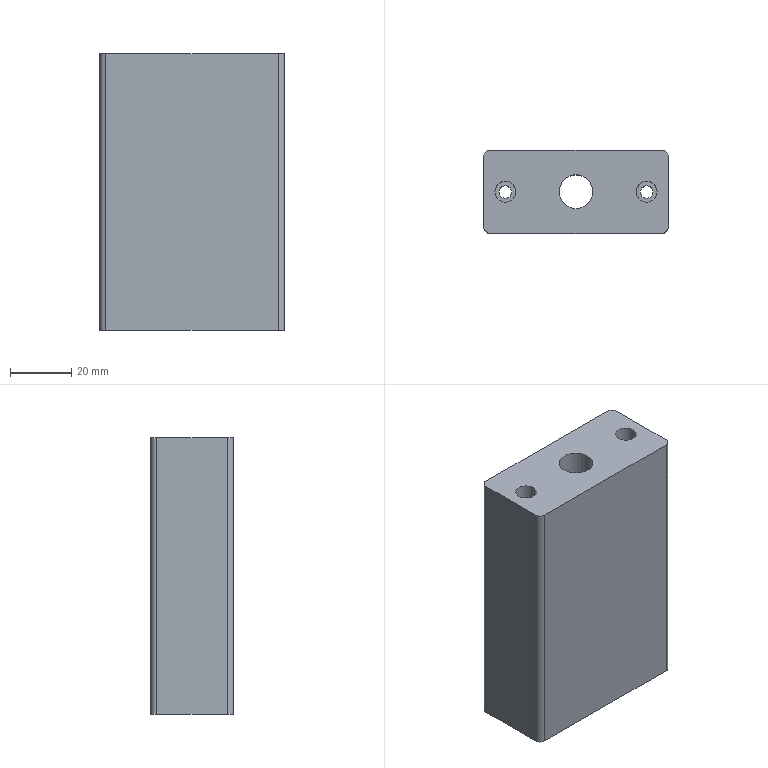Part | STEP file | gslz 2016.10.28-10_id2870_x_t | 1 solid | 19 faces | box 60 x 27 x 90 mm | volume 122829 mm3 | cylinder 10 | plane 9 | commonest cylinder face diameters 4 x4 4.1 x2 6.8 x2 11 x1 17 x1
STEP:
#1=CARTESIAN_POINT('',(0.,0.,0.));
#2=DIRECTION('',(0.,0.,1.));
#3=DIRECTION('',(1.,0.,0.));
#4=AXIS2_PLACEMENT_3D('',#1,#2,#3);
#5=CARTESIAN_POINT('',(1032.,147.5,85.));
#6=VERTEX_POINT('',#5);
#7=CARTESIAN_POINT('',(1088.,147.5,85.));
#8=VERTEX_POINT('',#7);
#9=CARTESIAN_POINT('',(1170.635,147.5,85.));
#10=DIRECTION('',(1.,0.,0.));
#11=VECTOR('',#10,1.);
#12=LINE('',#9,#11);
#13=CARTESIAN_POINT('',(1128.,155.,85.));
#14=DIRECTION('',(0.,0.,1.));
#15=DIRECTION('',(-1.,0.,0.));
#16=AXIS2_PLACEMENT_3D('',#13,#14,#15);
#17=PLANE('',#16);
#18=CARTESIAN_POINT('',(-42.635,7.5));
#19=DIRECTION('',(-1.,0.));
#20=VECTOR('',#19,1.);
#21=LINE('',#18,#20);
#22=(GEOMETRIC_REPRESENTATION_CONTEXT(2)PARAMETRIC_REPRESENTATION_CONTEXT()REPRESENTATION_CONTEXT('',''));
#23=DEFINITIONAL_REPRESENTATION('',(#21),#22);
#24=PCURVE('',#17,#23);
#25=CARTESIAN_POINT('',(1170.635,147.5,80.));
#26=DIRECTION('',(0.,1.,0.));
#27=DIRECTION('',(0.,0.,-1.));
#28=AXIS2_PLACEMENT_3D('',#25,#26,#27);
#29=PLANE('',#28);
#30=CARTESIAN_POINT('',(-5.,0.));
#31=DIRECTION('',(0.,-1.));
#32=VECTOR('',#31,1.);
#33=LINE('',#30,#32);
#34=(GEOMETRIC_REPRESENTATION_CONTEXT(2)PARAMETRIC_REPRESENTATION_CONTEXT()REPRESENTATION_CONTEXT('',''));
#35=DEFINITIONAL_REPRESENTATION('',(#33),#34);
#36=PCURVE('',#29,#35);
#37=SURFACE_CURVE('',#12,(#24,#36),.PCURVE_S1.);
#38=EDGE_CURVE('',#6,#8,#37,.T.);
#39=ORIENTED_EDGE('',*,*,#38,.T.);
#40=CARTESIAN_POINT('',(1090.,149.5,85.));
#41=VERTEX_POINT('',#40);
#42=CARTESIAN_POINT('',(1088.,149.5,85.));
#43=DIRECTION('',(0.,0.,1.));
#44=DIRECTION('',(1.,0.,0.));
#45=AXIS2_PLACEMENT_3D('',#42,#43,#44);
#46=CIRCLE('',#45,2.);
#47=CARTESIAN_POINT('',(40.,5.5));
#48=DIRECTION('',(-1.,0.));
#49=AXIS2_PLACEMENT_2D('',#47,#48);
#50=CIRCLE('',#49,2.);
#51=(GEOMETRIC_REPRESENTATION_CONTEXT(2)PARAMETRIC_REPRESENTATION_CONTEXT()REPRESENTATION_CONTEXT('',''));
#52=DEFINITIONAL_REPRESENTATION('',(#50),#51);
#53=PCURVE('',#17,#52);
#54=CARTESIAN_POINT('',(1088.,149.5,80.));
#55=DIRECTION('',(0.,0.,1.));
#56=DIRECTION('',(-1.,0.,0.));
#57=AXIS2_PLACEMENT_3D('',#54,#55,#56);
#58=CYLINDRICAL_SURFACE('',#57,2.);
#59=CARTESIAN_POINT('',(-3.142,5.));
#60=DIRECTION('',(1.,0.));
#61=VECTOR('',#60,1.);
#62=LINE('',#59,#61);
#63=(GEOMETRIC_REPRESENTATION_CONTEXT(2)PARAMETRIC_REPRESENTATION_CONTEXT()REPRESENTATION_CONTEXT('',''));
#64=DEFINITIONAL_REPRESENTATION('',(#62),#63);
#65=PCURVE('',#58,#64);
#66=SURFACE_CURVE('',#46,(#53,#65),.PCURVE_S1.);
#67=EDGE_CURVE('',#8,#41,#66,.T.);
#68=ORIENTED_EDGE('',*,*,#67,.T.);
#69=CARTESIAN_POINT('',(1090.,172.5,85.));
#70=VERTEX_POINT('',#69);
#71=CARTESIAN_POINT('',(1090.,161.,85.));
#72=DIRECTION('',(0.,1.,0.));
#73=VECTOR('',#72,1.);
#74=LINE('',#71,#73);
#75=CARTESIAN_POINT('',(38.,-6.));
#76=DIRECTION('',(0.,-1.));
#77=VECTOR('',#76,1.);
#78=LINE('',#75,#77);
#79=(GEOMETRIC_REPRESENTATION_CONTEXT(2)PARAMETRIC_REPRESENTATION_CONTEXT()REPRESENTATION_CONTEXT('',''));
#80=DEFINITIONAL_REPRESENTATION('',(#78),#79);
#81=PCURVE('',#17,#80);
#82=CARTESIAN_POINT('',(1090.,161.,46.));
#83=DIRECTION('',(-1.,0.,0.));
#84=DIRECTION('',(0.,0.,-1.));
#85=AXIS2_PLACEMENT_3D('',#82,#83,#84);
#86=PLANE('',#85);
#87=CARTESIAN_POINT('',(-39.,0.));
#88=DIRECTION('',(0.,-1.));
#89=VECTOR('',#88,1.);
#90=LINE('',#87,#89);
#91=(GEOMETRIC_REPRESENTATION_CONTEXT(2)PARAMETRIC_REPRESENTATION_CONTEXT()REPRESENTATION_CONTEXT('',''));
#92=DEFINITIONAL_REPRESENTATION('',(#90),#91);
#93=PCURVE('',#86,#92);
#94=SURFACE_CURVE('',#74,(#81,#93),.PCURVE_S1.);
#95=EDGE_CURVE('',#41,#70,#94,.T.);
#96=ORIENTED_EDGE('',*,*,#95,.T.);
#97=CARTESIAN_POINT('',(1088.,174.5,85.));
#98=VERTEX_POINT('',#97);
#99=CARTESIAN_POINT('',(1088.,172.5,85.));
#100=DIRECTION('',(0.,0.,1.));
#101=DIRECTION('',(1.,0.,0.));
#102=AXIS2_PLACEMENT_3D('',#99,#100,#101);
#103=CIRCLE('',#102,2.);
#104=CARTESIAN_POINT('',(40.,-17.5));
#105=DIRECTION('',(-1.,0.));
#106=AXIS2_PLACEMENT_2D('',#104,#105);
#107=CIRCLE('',#106,2.);
#108=(GEOMETRIC_REPRESENTATION_CONTEXT(2)PARAMETRIC_REPRESENTATION_CONTEXT()REPRESENTATION_CONTEXT('',''));
#109=DEFINITIONAL_REPRESENTATION('',(#107),#108);
#110=PCURVE('',#17,#109);
#111=CARTESIAN_POINT('',(1088.,172.5,46.));
#112=DIRECTION('',(0.,0.,1.));
#113=DIRECTION('',(-1.,0.,0.));
#114=AXIS2_PLACEMENT_3D('',#111,#112,#113);
#115=CYLINDRICAL_SURFACE('',#114,2.);
#116=CARTESIAN_POINT('',(-3.142,39.));
#117=DIRECTION('',(1.,0.));
#118=VECTOR('',#117,1.);
#119=LINE('',#116,#118);
#120=(GEOMETRIC_REPRESENTATION_CONTEXT(2)PARAMETRIC_REPRESENTATION_CONTEXT()REPRESENTATION_CONTEXT('',''));
#121=DEFINITIONAL_REPRESENTATION('',(#119),#120);
#122=PCURVE('',#115,#121);
#123=SURFACE_CURVE('',#103,(#110,#122),.PCURVE_S1.);
#124=EDGE_CURVE('',#70,#98,#123,.T.);
#125=ORIENTED_EDGE('',*,*,#124,.T.);
#126=CARTESIAN_POINT('',(1032.,174.5,85.));
#127=VERTEX_POINT('',#126);
#128=CARTESIAN_POINT('',(435.,174.5,85.));
#129=DIRECTION('',(-1.,0.,0.));
#130=VECTOR('',#129,1.);
#131=LINE('',#128,#130);
#132=CARTESIAN_POINT('',(693.,-19.5));
#133=DIRECTION('',(1.,0.));
#134=VECTOR('',#133,1.);
#135=LINE('',#132,#134);
#136=(GEOMETRIC_REPRESENTATION_CONTEXT(2)PARAMETRIC_REPRESENTATION_CONTEXT()REPRESENTATION_CONTEXT('',''));
#137=DEFINITIONAL_REPRESENTATION('',(#135),#136);
#138=PCURVE('',#17,#137);
#139=CARTESIAN_POINT('',(435.,174.5,80.));
#140=DIRECTION('',(0.,-1.,0.));
#141=DIRECTION('',(0.,0.,1.));
#142=AXIS2_PLACEMENT_3D('',#139,#140,#141);
#143=PLANE('',#142);
#144=CARTESIAN_POINT('',(5.,0.));
#145=DIRECTION('',(0.,1.));
#146=VECTOR('',#145,1.);
#147=LINE('',#144,#146);
#148=(GEOMETRIC_REPRESENTATION_CONTEXT(2)PARAMETRIC_REPRESENTATION_CONTEXT()REPRESENTATION_CONTEXT('',''));
#149=DEFINITIONAL_REPRESENTATION('',(#147),#148);
#150=PCURVE('',#143,#149);
#151=SURFACE_CURVE('',#131,(#138,#150),.PCURVE_S1.);
#152=EDGE_CURVE('',#98,#127,#151,.T.);
#153=ORIENTED_EDGE('',*,*,#152,.T.);
#154=CARTESIAN_POINT('',(1030.,172.5,85.));
#155=VERTEX_POINT('',#154);
#156=CARTESIAN_POINT('',(1032.,172.5,85.));
#157=DIRECTION('',(0.,0.,1.));
#158=DIRECTION('',(1.,0.,0.));
#159=AXIS2_PLACEMENT_3D('',#156,#157,#158);
#160=CIRCLE('',#159,2.);
#161=CARTESIAN_POINT('',(96.,-17.5));
#162=DIRECTION('',(-1.,0.));
#163=AXIS2_PLACEMENT_2D('',#161,#162);
#164=CIRCLE('',#163,2.);
#165=(GEOMETRIC_REPRESENTATION_CONTEXT(2)PARAMETRIC_REPRESENTATION_CONTEXT()REPRESENTATION_CONTEXT('',''));
#166=DEFINITIONAL_REPRESENTATION('',(#164),#165);
#167=PCURVE('',#17,#166);
#168=CARTESIAN_POINT('',(1032.,172.5,80.));
#169=DIRECTION('',(0.,0.,1.));
#170=DIRECTION('',(-1.,0.,0.));
#171=AXIS2_PLACEMENT_3D('',#168,#169,#170);
#172=CYLINDRICAL_SURFACE('',#171,2.);
#173=CARTESIAN_POINT('',(3.142,5.));
#174=DIRECTION('',(1.,0.));
#175=VECTOR('',#174,1.);
#176=LINE('',#173,#175);
#177=(GEOMETRIC_REPRESENTATION_CONTEXT(2)PARAMETRIC_REPRESENTATION_CONTEXT()REPRESENTATION_CONTEXT('',''));
#178=DEFINITIONAL_REPRESENTATION('',(#176),#177);
#179=PCURVE('',#172,#178);
#180=SURFACE_CURVE('',#160,(#167,#179),.PCURVE_S1.);
#181=EDGE_CURVE('',#127,#155,#180,.T.);
#182=ORIENTED_EDGE('',*,*,#181,.T.);
#183=CARTESIAN_POINT('',(1030.,149.5,85.));
#184=VERTEX_POINT('',#183);
#185=CARTESIAN_POINT('',(1030.,167.5,85.));
#186=DIRECTION('',(0.,1.,0.));
#187=VECTOR('',#186,1.);
#188=LINE('',#185,#187);
#189=CARTESIAN_POINT('',(98.,-12.5));
#190=DIRECTION('',(0.,-1.));
#191=VECTOR('',#190,1.);
#192=LINE('',#189,#191);
#193=(GEOMETRIC_REPRESENTATION_CONTEXT(2)PARAMETRIC_REPRESENTATION_CONTEXT()REPRESENTATION_CONTEXT('',''));
#194=DEFINITIONAL_REPRESENTATION('',(#192),#193);
#195=PCURVE('',#17,#194);
#196=CARTESIAN_POINT('',(1030.,167.5,80.));
#197=DIRECTION('',(-1.,0.,0.));
#198=DIRECTION('',(0.,0.,-1.));
#199=AXIS2_PLACEMENT_3D('',#196,#197,#198);
#200=PLANE('',#199);
#201=CARTESIAN_POINT('',(-5.,0.));
#202=DIRECTION('',(0.,-1.));
#203=VECTOR('',#202,1.);
#204=LINE('',#201,#203);
#205=(GEOMETRIC_REPRESENTATION_CONTEXT(2)PARAMETRIC_REPRESENTATION_CONTEXT()REPRESENTATION_CONTEXT('',''));
#206=DEFINITIONAL_REPRESENTATION('',(#204),#205);
#207=PCURVE('',#200,#206);
#208=SURFACE_CURVE('',#188,(#195,#207),.PCURVE_S1.);
#209=EDGE_CURVE('',#184,#155,#208,.T.);
#210=ORIENTED_EDGE('',*,*,#209,.F.);
#211=CARTESIAN_POINT('',(1032.,149.5,85.));
#212=DIRECTION('',(0.,0.,1.));
#213=DIRECTION('',(1.,0.,0.));
#214=AXIS2_PLACEMENT_3D('',#211,#212,#213);
#215=CIRCLE('',#214,2.);
#216=CARTESIAN_POINT('',(96.,5.5));
#217=DIRECTION('',(-1.,0.));
#218=AXIS2_PLACEMENT_2D('',#216,#217);
#219=CIRCLE('',#218,2.);
#220=(GEOMETRIC_REPRESENTATION_CONTEXT(2)PARAMETRIC_REPRESENTATION_CONTEXT()REPRESENTATION_CONTEXT('',''));
#221=DEFINITIONAL_REPRESENTATION('',(#219),#220);
#222=PCURVE('',#17,#221);
#223=CARTESIAN_POINT('',(1032.,149.5,80.));
#224=DIRECTION('',(0.,0.,1.));
#225=DIRECTION('',(-1.,0.,0.));
#226=AXIS2_PLACEMENT_3D('',#223,#224,#225);
#227=CYLINDRICAL_SURFACE('',#226,2.);
#228=CARTESIAN_POINT('',(-3.142,5.));
#229=DIRECTION('',(1.,0.));
#230=VECTOR('',#229,1.);
#231=LINE('',#228,#230);
#232=(GEOMETRIC_REPRESENTATION_CONTEXT(2)PARAMETRIC_REPRESENTATION_CONTEXT()REPRESENTATION_CONTEXT('',''));
#233=DEFINITIONAL_REPRESENTATION('',(#231),#232);
#234=PCURVE('',#227,#233);
#235=SURFACE_CURVE('',#215,(#222,#234),.PCURVE_S1.);
#236=EDGE_CURVE('',#184,#6,#235,.T.);
#237=ORIENTED_EDGE('',*,*,#236,.T.);
#238=EDGE_LOOP('',(#39,#68,#96,#125,#153,#182,#210,#237));
#239=FACE_BOUND('',#238,.T.);
#240=CARTESIAN_POINT('',(1065.5,161.,85.));
#241=VERTEX_POINT('',#240);
#242=CARTESIAN_POINT('',(1060.,161.,85.));
#243=DIRECTION('',(0.,0.,1.));
#244=DIRECTION('',(1.,0.,0.));
#245=AXIS2_PLACEMENT_3D('',#242,#243,#244);
#246=CIRCLE('',#245,5.5);
#247=CARTESIAN_POINT('',(68.,-6.));
#248=DIRECTION('',(-1.,0.));
#249=AXIS2_PLACEMENT_2D('',#247,#248);
#250=CIRCLE('',#249,5.5);
#251=(GEOMETRIC_REPRESENTATION_CONTEXT(2)PARAMETRIC_REPRESENTATION_CONTEXT()REPRESENTATION_CONTEXT('',''));
#252=DEFINITIONAL_REPRESENTATION('',(#250),#251);
#253=PCURVE('',#17,#252);
#254=CARTESIAN_POINT('',(1060.,161.,-13.));
#255=DIRECTION('',(0.,0.,1.));
#256=DIRECTION('',(1.,0.,0.));
#257=AXIS2_PLACEMENT_3D('',#254,#255,#256);
#258=CYLINDRICAL_SURFACE('',#257,5.5);
#259=CARTESIAN_POINT('',(0.,98.));
#260=DIRECTION('',(1.,0.));
#261=VECTOR('',#260,1.);
#262=LINE('',#259,#261);
#263=(GEOMETRIC_REPRESENTATION_CONTEXT(2)PARAMETRIC_REPRESENTATION_CONTEXT()REPRESENTATION_CONTEXT('',''));
#264=DEFINITIONAL_REPRESENTATION('',(#262),#263);
#265=PCURVE('',#258,#264);
#266=SURFACE_CURVE('',#246,(#253,#265),.PCURVE_S1.);
#267=EDGE_CURVE('',#241,#241,#266,.T.);
#268=ORIENTED_EDGE('',*,*,#267,.F.);
#269=EDGE_LOOP('',(#268));
#270=FACE_BOUND('',#269,.T.);
#271=CARTESIAN_POINT('',(1033.6,161.,85.));
#272=VERTEX_POINT('',#271);
#273=CARTESIAN_POINT('',(1037.,161.,85.));
#274=DIRECTION('',(0.,0.,1.));
#275=DIRECTION('',(-1.,0.,0.));
#276=AXIS2_PLACEMENT_3D('',#273,#274,#275);
#277=CIRCLE('',#276,3.4);
#278=CARTESIAN_POINT('',(91.,-6.));
#279=DIRECTION('',(1.,0.));
#280=AXIS2_PLACEMENT_2D('',#278,#279);
#281=CIRCLE('',#280,3.4);
#282=(GEOMETRIC_REPRESENTATION_CONTEXT(2)PARAMETRIC_REPRESENTATION_CONTEXT()REPRESENTATION_CONTEXT('',''));
#283=DEFINITIONAL_REPRESENTATION('',(#281),#282);
#284=PCURVE('',#17,#283);
#285=CARTESIAN_POINT('',(1037.,161.,31.));
#286=DIRECTION('',(0.,0.,1.));
#287=DIRECTION('',(1.,0.,0.));
#288=AXIS2_PLACEMENT_3D('',#285,#286,#287);
#289=CYLINDRICAL_SURFACE('',#288,3.4);
#290=CARTESIAN_POINT('',(3.142,54.));
#291=DIRECTION('',(1.,0.));
#292=VECTOR('',#291,1.);
#293=LINE('',#290,#292);
#294=(GEOMETRIC_REPRESENTATION_CONTEXT(2)PARAMETRIC_REPRESENTATION_CONTEXT()REPRESENTATION_CONTEXT('',''));
#295=DEFINITIONAL_REPRESENTATION('',(#293),#294);
#296=PCURVE('',#289,#295);
#297=SURFACE_CURVE('',#277,(#284,#296),.PCURVE_S1.);
#298=EDGE_CURVE('',#272,#272,#297,.T.);
#299=ORIENTED_EDGE('',*,*,#298,.F.);
#300=EDGE_LOOP('',(#299));
#301=FACE_BOUND('',#300,.T.);
#302=CARTESIAN_POINT('',(1086.4,161.,85.));
#303=VERTEX_POINT('',#302);
#304=CARTESIAN_POINT('',(1083.,161.,85.));
#305=DIRECTION('',(0.,0.,-1.));
#306=DIRECTION('',(1.,0.,0.));
#307=AXIS2_PLACEMENT_3D('',#304,#305,#306);
#308=CIRCLE('',#307,3.4);
#309=CARTESIAN_POINT('',(41.6,-6.));
#310=CARTESIAN_POINT('',(41.6,-0.111));
#311=CARTESIAN_POINT('',(46.7,-3.056));
#312=CARTESIAN_POINT('',(51.8,-6.));
#313=CARTESIAN_POINT('',(46.7,-8.944));
#314=CARTESIAN_POINT('',(41.6,-11.889));
#315=CARTESIAN_POINT('',(41.6,-6.));
#316=(BOUNDED_CURVE()B_SPLINE_CURVE(2,(#309,#310,#311,#312,#313,#314,#315),.UNSPECIFIED.,.T.,.F.)B_SPLINE_CURVE_WITH_KNOTS((1,2,2,2,2,1),(-2.094,0.,2.094,4.189,6.283,8.378),.UNSPECIFIED.)CURVE()GEOMETRIC_REPRESENTATION_ITEM()RATIONAL_B_SPLINE_CURVE((1.,0.5,1.,0.5,1.,0.5,1.))REPRESENTATION_ITEM(''));
#317=(GEOMETRIC_REPRESENTATION_CONTEXT(2)PARAMETRIC_REPRESENTATION_CONTEXT()REPRESENTATION_CONTEXT('',''));
#318=DEFINITIONAL_REPRESENTATION('',(#316),#317);
#319=PCURVE('',#17,#318);
#320=CARTESIAN_POINT('',(1083.,161.,31.));
#321=DIRECTION('',(0.,0.,1.));
#322=DIRECTION('',(-1.,0.,0.));
#323=AXIS2_PLACEMENT_3D('',#320,#321,#322);
#324=CYLINDRICAL_SURFACE('',#323,3.4);
#325=CARTESIAN_POINT('',(9.425,54.));
#326=DIRECTION('',(-1.,0.));
#327=VECTOR('',#326,1.);
#328=LINE('',#325,#327);
#329=(GEOMETRIC_REPRESENTATION_CONTEXT(2)PARAMETRIC_REPRESENTATION_CONTEXT()REPRESENTATION_CONTEXT('',''));
#330=DEFINITIONAL_REPRESENTATION('',(#328),#329);
#331=PCURVE('',#324,#330);
#332=SURFACE_CURVE('',#308,(#319,#331),.PCURVE_S1.);
#333=EDGE_CURVE('',#303,#303,#332,.T.);
#334=ORIENTED_EDGE('',*,*,#333,.T.);
#335=EDGE_LOOP('',(#334));
#336=FACE_BOUND('',#335,.T.);
#337=ADVANCED_FACE('',(#239,#270,#301,#336),#17,.T.);
#338=CARTESIAN_POINT('',(1080.95,161.,-5.));
#339=VERTEX_POINT('',#338);
#340=CARTESIAN_POINT('',(1083.,161.,-5.));
#341=DIRECTION('',(0.,0.,1.));
#342=DIRECTION('',(-1.,0.,0.));
#343=AXIS2_PLACEMENT_3D('',#340,#341,#342);
#344=CIRCLE('',#343,2.05);
#345=CARTESIAN_POINT('',(439.5,67.646,-5.));
#346=DIRECTION('',(0.,0.,-1.));
#347=DIRECTION('',(1.,0.,0.));
#348=AXIS2_PLACEMENT_3D('',#345,#346,#347);
#349=PLANE('',#348);
#350=CARTESIAN_POINT('',(641.45,-93.354));
#351=CARTESIAN_POINT('',(641.45,-89.804));
#352=CARTESIAN_POINT('',(644.525,-91.579));
#353=CARTESIAN_POINT('',(647.6,-93.354));
#354=CARTESIAN_POINT('',(644.525,-95.13));
#355=CARTESIAN_POINT('',(641.45,-96.905));
#356=CARTESIAN_POINT('',(641.45,-93.354));
#357=(BOUNDED_CURVE()B_SPLINE_CURVE(2,(#350,#351,#352,#353,#354,#355,#356),.UNSPECIFIED.,.T.,.F.)B_SPLINE_CURVE_WITH_KNOTS((1,2,2,2,2,1),(-2.094,0.,2.094,4.189,6.283,8.378),.UNSPECIFIED.)CURVE()GEOMETRIC_REPRESENTATION_ITEM()RATIONAL_B_SPLINE_CURVE((1.,0.5,1.,0.5,1.,0.5,1.))REPRESENTATION_ITEM(''));
#358=(GEOMETRIC_REPRESENTATION_CONTEXT(2)PARAMETRIC_REPRESENTATION_CONTEXT()REPRESENTATION_CONTEXT('',''));
#359=DEFINITIONAL_REPRESENTATION('',(#357),#358);
#360=PCURVE('',#349,#359);
#361=CARTESIAN_POINT('',(1083.,161.,36.));
#362=DIRECTION('',(0.,0.,-1.));
#363=DIRECTION('',(1.,0.,0.));
#364=AXIS2_PLACEMENT_3D('',#361,#362,#363);
#365=CYLINDRICAL_SURFACE('',#364,2.05);
#366=CARTESIAN_POINT('',(9.425,41.));
#367=DIRECTION('',(-1.,0.));
#368=VECTOR('',#367,1.);
#369=LINE('',#366,#368);
#370=(GEOMETRIC_REPRESENTATION_CONTEXT(2)PARAMETRIC_REPRESENTATION_CONTEXT()REPRESENTATION_CONTEXT('',''));
#371=DEFINITIONAL_REPRESENTATION('',(#369),#370);
#372=PCURVE('',#365,#371);
#373=SURFACE_CURVE('',#344,(#360,#372),.PCURVE_S1.);
#374=EDGE_CURVE('',#339,#339,#373,.T.);
#375=ORIENTED_EDGE('',*,*,#374,.T.);
#376=EDGE_LOOP('',(#375));
#377=FACE_BOUND('',#376,.T.);
#378=CARTESIAN_POINT('',(1034.95,161.,-5.));
#379=VERTEX_POINT('',#378);
#380=CARTESIAN_POINT('',(1037.,161.,-5.));
#381=DIRECTION('',(0.,0.,1.));
#382=DIRECTION('',(-1.,0.,0.));
#383=AXIS2_PLACEMENT_3D('',#380,#381,#382);
#384=CIRCLE('',#383,2.05);
#385=CARTESIAN_POINT('',(595.45,-93.354));
#386=CARTESIAN_POINT('',(595.45,-89.804));
#387=CARTESIAN_POINT('',(598.525,-91.579));
#388=CARTESIAN_POINT('',(601.6,-93.354));
#389=CARTESIAN_POINT('',(598.525,-95.13));
#390=CARTESIAN_POINT('',(595.45,-96.905));
#391=CARTESIAN_POINT('',(595.45,-93.354));
#392=(BOUNDED_CURVE()B_SPLINE_CURVE(2,(#385,#386,#387,#388,#389,#390,#391),.UNSPECIFIED.,.T.,.F.)B_SPLINE_CURVE_WITH_KNOTS((1,2,2,2,2,1),(-2.094,0.,2.094,4.189,6.283,8.378),.UNSPECIFIED.)CURVE()GEOMETRIC_REPRESENTATION_ITEM()RATIONAL_B_SPLINE_CURVE((1.,0.5,1.,0.5,1.,0.5,1.))REPRESENTATION_ITEM(''));
#393=(GEOMETRIC_REPRESENTATION_CONTEXT(2)PARAMETRIC_REPRESENTATION_CONTEXT()REPRESENTATION_CONTEXT('',''));
#394=DEFINITIONAL_REPRESENTATION('',(#392),#393);
#395=PCURVE('',#349,#394);
#396=CARTESIAN_POINT('',(1037.,161.,36.));
#397=DIRECTION('',(0.,0.,-1.));
#398=DIRECTION('',(-1.,0.,0.));
#399=AXIS2_PLACEMENT_3D('',#396,#397,#398);
#400=CYLINDRICAL_SURFACE('',#399,2.05);
#401=CARTESIAN_POINT('',(6.283,41.));
#402=DIRECTION('',(-1.,0.));
#403=VECTOR('',#402,1.);
#404=LINE('',#401,#403);
#405=(GEOMETRIC_REPRESENTATION_CONTEXT(2)PARAMETRIC_REPRESENTATION_CONTEXT()REPRESENTATION_CONTEXT('',''));
#406=DEFINITIONAL_REPRESENTATION('',(#404),#405);
#407=PCURVE('',#400,#406);
#408=SURFACE_CURVE('',#384,(#395,#407),.PCURVE_S1.);
#409=EDGE_CURVE('',#379,#379,#408,.T.);
#410=ORIENTED_EDGE('',*,*,#409,.T.);
#411=EDGE_LOOP('',(#410));
#412=FACE_BOUND('',#411,.T.);
#413=CARTESIAN_POINT('',(1090.,172.5,-5.));
#414=VERTEX_POINT('',#413);
#415=CARTESIAN_POINT('',(1090.,149.5,-5.));
#416=VERTEX_POINT('',#415);
#417=CARTESIAN_POINT('',(1090.,161.,-5.));
#418=DIRECTION('',(0.,-1.,0.));
#419=VECTOR('',#418,1.);
#420=LINE('',#417,#419);
#421=CARTESIAN_POINT('',(650.5,-93.354));
#422=DIRECTION('',(0.,1.));
#423=VECTOR('',#422,1.);
#424=LINE('',#421,#423);
#425=(GEOMETRIC_REPRESENTATION_CONTEXT(2)PARAMETRIC_REPRESENTATION_CONTEXT()REPRESENTATION_CONTEXT('',''));
#426=DEFINITIONAL_REPRESENTATION('',(#424),#425);
#427=PCURVE('',#349,#426);
#428=CARTESIAN_POINT('',(51.,0.));
#429=DIRECTION('',(0.,1.));
#430=VECTOR('',#429,1.);
#431=LINE('',#428,#430);
#432=(GEOMETRIC_REPRESENTATION_CONTEXT(2)PARAMETRIC_REPRESENTATION_CONTEXT()REPRESENTATION_CONTEXT('',''));
#433=DEFINITIONAL_REPRESENTATION('',(#431),#432);
#434=PCURVE('',#86,#433);
#435=SURFACE_CURVE('',#420,(#427,#434),.PCURVE_S1.);
#436=EDGE_CURVE('',#414,#416,#435,.T.);
#437=ORIENTED_EDGE('',*,*,#436,.T.);
#438=CARTESIAN_POINT('',(1088.,147.5,-5.));
#439=VERTEX_POINT('',#438);
#440=CARTESIAN_POINT('',(1088.,149.5,-5.));
#441=DIRECTION('',(0.,0.,-1.));
#442=DIRECTION('',(-1.,0.,0.));
#443=AXIS2_PLACEMENT_3D('',#440,#441,#442);
#444=CIRCLE('',#443,2.);
#445=CARTESIAN_POINT('',(648.5,-81.854));
#446=DIRECTION('',(-1.,0.));
#447=AXIS2_PLACEMENT_2D('',#445,#446);
#448=CIRCLE('',#447,2.);
#449=(GEOMETRIC_REPRESENTATION_CONTEXT(2)PARAMETRIC_REPRESENTATION_CONTEXT()REPRESENTATION_CONTEXT('',''));
#450=DEFINITIONAL_REPRESENTATION('',(#448),#449);
#451=PCURVE('',#349,#450);
#452=CARTESIAN_POINT('',(6.283,-85.));
#453=DIRECTION('',(-1.,0.));
#454=VECTOR('',#453,1.);
#455=LINE('',#452,#454);
#456=(GEOMETRIC_REPRESENTATION_CONTEXT(2)PARAMETRIC_REPRESENTATION_CONTEXT()REPRESENTATION_CONTEXT('',''));
#457=DEFINITIONAL_REPRESENTATION('',(#455),#456);
#458=PCURVE('',#58,#457);
#459=SURFACE_CURVE('',#444,(#451,#458),.PCURVE_S1.);
#460=EDGE_CURVE('',#416,#439,#459,.T.);
#461=ORIENTED_EDGE('',*,*,#460,.T.);
#462=CARTESIAN_POINT('',(1032.,147.5,-5.));
#463=VERTEX_POINT('',#462);
#464=CARTESIAN_POINT('',(439.5,147.5,-5.));
#465=DIRECTION('',(1.,0.,0.));
#466=VECTOR('',#465,1.);
#467=LINE('',#464,#466);
#468=CARTESIAN_POINT('',(0.,-79.854));
#469=DIRECTION('',(1.,0.));
#470=VECTOR('',#469,1.);
#471=LINE('',#468,#470);
#472=(GEOMETRIC_REPRESENTATION_CONTEXT(2)PARAMETRIC_REPRESENTATION_CONTEXT()REPRESENTATION_CONTEXT('',''));
#473=DEFINITIONAL_REPRESENTATION('',(#471),#472);
#474=PCURVE('',#349,#473);
#475=CARTESIAN_POINT('',(85.,731.135));
#476=DIRECTION('',(0.,-1.));
#477=VECTOR('',#476,1.);
#478=LINE('',#475,#477);
#479=(GEOMETRIC_REPRESENTATION_CONTEXT(2)PARAMETRIC_REPRESENTATION_CONTEXT()REPRESENTATION_CONTEXT('',''));
#480=DEFINITIONAL_REPRESENTATION('',(#478),#479);
#481=PCURVE('',#29,#480);
#482=SURFACE_CURVE('',#467,(#474,#481),.PCURVE_S1.);
#483=EDGE_CURVE('',#463,#439,#482,.T.);
#484=ORIENTED_EDGE('',*,*,#483,.F.);
#485=CARTESIAN_POINT('',(1030.,149.5,-5.));
#486=VERTEX_POINT('',#485);
#487=CARTESIAN_POINT('',(1032.,149.5,-5.));
#488=DIRECTION('',(0.,0.,-1.));
#489=DIRECTION('',(-1.,0.,0.));
#490=AXIS2_PLACEMENT_3D('',#487,#488,#489);
#491=CIRCLE('',#490,2.);
#492=CARTESIAN_POINT('',(592.5,-81.854));
#493=DIRECTION('',(-1.,0.));
#494=AXIS2_PLACEMENT_2D('',#492,#493);
#495=CIRCLE('',#494,2.);
#496=(GEOMETRIC_REPRESENTATION_CONTEXT(2)PARAMETRIC_REPRESENTATION_CONTEXT()REPRESENTATION_CONTEXT('',''));
#497=DEFINITIONAL_REPRESENTATION('',(#495),#496);
#498=PCURVE('',#349,#497);
#499=CARTESIAN_POINT('',(6.283,-85.));
#500=DIRECTION('',(-1.,0.));
#501=VECTOR('',#500,1.);
#502=LINE('',#499,#501);
#503=(GEOMETRIC_REPRESENTATION_CONTEXT(2)PARAMETRIC_REPRESENTATION_CONTEXT()REPRESENTATION_CONTEXT('',''));
#504=DEFINITIONAL_REPRESENTATION('',(#502),#503);
#505=PCURVE('',#227,#504);
#506=SURFACE_CURVE('',#491,(#498,#505),.PCURVE_S1.);
#507=EDGE_CURVE('',#463,#486,#506,.T.);
#508=ORIENTED_EDGE('',*,*,#507,.T.);
#509=CARTESIAN_POINT('',(1030.,172.5,-5.));
#510=VERTEX_POINT('',#509);
#511=CARTESIAN_POINT('',(1030.,67.646,-5.));
#512=DIRECTION('',(0.,1.,0.));
#513=VECTOR('',#512,1.);
#514=LINE('',#511,#513);
#515=CARTESIAN_POINT('',(590.5,0.));
#516=DIRECTION('',(0.,-1.));
#517=VECTOR('',#516,1.);
#518=LINE('',#515,#517);
#519=(GEOMETRIC_REPRESENTATION_CONTEXT(2)PARAMETRIC_REPRESENTATION_CONTEXT()REPRESENTATION_CONTEXT('',''));
#520=DEFINITIONAL_REPRESENTATION('',(#518),#519);
#521=PCURVE('',#349,#520);
#522=CARTESIAN_POINT('',(85.,99.854));
#523=DIRECTION('',(0.,-1.));
#524=VECTOR('',#523,1.);
#525=LINE('',#522,#524);
#526=(GEOMETRIC_REPRESENTATION_CONTEXT(2)PARAMETRIC_REPRESENTATION_CONTEXT()REPRESENTATION_CONTEXT('',''));
#527=DEFINITIONAL_REPRESENTATION('',(#525),#526);
#528=PCURVE('',#200,#527);
#529=SURFACE_CURVE('',#514,(#521,#528),.PCURVE_S1.);
#530=EDGE_CURVE('',#486,#510,#529,.T.);
#531=ORIENTED_EDGE('',*,*,#530,.T.);
#532=CARTESIAN_POINT('',(1032.,174.5,-5.));
#533=VERTEX_POINT('',#532);
#534=CARTESIAN_POINT('',(1032.,172.5,-5.));
#535=DIRECTION('',(0.,0.,-1.));
#536=DIRECTION('',(-1.,0.,0.));
#537=AXIS2_PLACEMENT_3D('',#534,#535,#536);
#538=CIRCLE('',#537,2.);
#539=CARTESIAN_POINT('',(592.5,-104.854));
#540=DIRECTION('',(-1.,0.));
#541=AXIS2_PLACEMENT_2D('',#539,#540);
#542=CIRCLE('',#541,2.);
#543=(GEOMETRIC_REPRESENTATION_CONTEXT(2)PARAMETRIC_REPRESENTATION_CONTEXT()REPRESENTATION_CONTEXT('',''));
#544=DEFINITIONAL_REPRESENTATION('',(#542),#543);
#545=PCURVE('',#349,#544);
#546=CARTESIAN_POINT('',(6.283,-85.));
#547=DIRECTION('',(-1.,0.));
#548=VECTOR('',#547,1.);
#549=LINE('',#546,#548);
#550=(GEOMETRIC_REPRESENTATION_CONTEXT(2)PARAMETRIC_REPRESENTATION_CONTEXT()REPRESENTATION_CONTEXT('',''));
#551=DEFINITIONAL_REPRESENTATION('',(#549),#550);
#552=PCURVE('',#172,#551);
#553=SURFACE_CURVE('',#538,(#545,#552),.PCURVE_S1.);
#554=EDGE_CURVE('',#510,#533,#553,.T.);
#555=ORIENTED_EDGE('',*,*,#554,.T.);
#556=CARTESIAN_POINT('',(1088.,174.5,-5.));
#557=VERTEX_POINT('',#556);
#558=CARTESIAN_POINT('',(439.5,174.5,-5.));
#559=DIRECTION('',(-1.,0.,0.));
#560=VECTOR('',#559,1.);
#561=LINE('',#558,#560);
#562=CARTESIAN_POINT('',(0.,-106.854));
#563=DIRECTION('',(-1.,0.));
#564=VECTOR('',#563,1.);
#565=LINE('',#562,#564);
#566=(GEOMETRIC_REPRESENTATION_CONTEXT(2)PARAMETRIC_REPRESENTATION_CONTEXT()REPRESENTATION_CONTEXT('',''));
#567=DEFINITIONAL_REPRESENTATION('',(#565),#566);
#568=PCURVE('',#349,#567);
#569=CARTESIAN_POINT('',(-85.,-4.5));
#570=DIRECTION('',(0.,1.));
#571=VECTOR('',#570,1.);
#572=LINE('',#569,#571);
#573=(GEOMETRIC_REPRESENTATION_CONTEXT(2)PARAMETRIC_REPRESENTATION_CONTEXT()REPRESENTATION_CONTEXT('',''));
#574=DEFINITIONAL_REPRESENTATION('',(#572),#573);
#575=PCURVE('',#143,#574);
#576=SURFACE_CURVE('',#561,(#568,#575),.PCURVE_S1.);
#577=EDGE_CURVE('',#557,#533,#576,.T.);
#578=ORIENTED_EDGE('',*,*,#577,.F.);
#579=CARTESIAN_POINT('',(1088.,172.5,-5.));
#580=DIRECTION('',(0.,0.,-1.));
#581=DIRECTION('',(-1.,0.,0.));
#582=AXIS2_PLACEMENT_3D('',#579,#580,#581);
#583=CIRCLE('',#582,2.);
#584=CARTESIAN_POINT('',(648.5,-104.854));
#585=DIRECTION('',(-1.,0.));
#586=AXIS2_PLACEMENT_2D('',#584,#585);
#587=CIRCLE('',#586,2.);
#588=(GEOMETRIC_REPRESENTATION_CONTEXT(2)PARAMETRIC_REPRESENTATION_CONTEXT()REPRESENTATION_CONTEXT('',''));
#589=DEFINITIONAL_REPRESENTATION('',(#587),#588);
#590=PCURVE('',#349,#589);
#591=CARTESIAN_POINT('',(6.283,-51.));
#592=DIRECTION('',(-1.,0.));
#593=VECTOR('',#592,1.);
#594=LINE('',#591,#593);
#595=(GEOMETRIC_REPRESENTATION_CONTEXT(2)PARAMETRIC_REPRESENTATION_CONTEXT()REPRESENTATION_CONTEXT('',''));
#596=DEFINITIONAL_REPRESENTATION('',(#594),#595);
#597=PCURVE('',#115,#596);
#598=SURFACE_CURVE('',#583,(#590,#597),.PCURVE_S1.);
#599=EDGE_CURVE('',#557,#414,#598,.T.);
#600=ORIENTED_EDGE('',*,*,#599,.T.);
#601=EDGE_LOOP('',(#437,#461,#484,#508,#531,#555,#578,#600));
#602=FACE_BOUND('',#601,.T.);
#603=CARTESIAN_POINT('',(1051.5,161.,-5.));
#604=VERTEX_POINT('',#603);
#605=CARTESIAN_POINT('',(1068.5,161.,-5.));
#606=VERTEX_POINT('',#605);
#607=CARTESIAN_POINT('',(1060.,161.,-5.));
#608=DIRECTION('',(0.,0.,-1.));
#609=DIRECTION('',(-1.,0.,0.));
#610=AXIS2_PLACEMENT_3D('',#607,#608,#609);
#611=CIRCLE('',#610,8.5);
#612=CARTESIAN_POINT('',(620.5,-93.354));
#613=DIRECTION('',(-1.,0.));
#614=AXIS2_PLACEMENT_2D('',#612,#613);
#615=CIRCLE('',#614,8.5);
#616=(GEOMETRIC_REPRESENTATION_CONTEXT(2)PARAMETRIC_REPRESENTATION_CONTEXT()REPRESENTATION_CONTEXT('',''));
#617=DEFINITIONAL_REPRESENTATION('',(#615),#616);
#618=PCURVE('',#349,#617);
#619=CARTESIAN_POINT('',(1060.,161.,-8.));
#620=DIRECTION('',(0.,0.,1.));
#621=DIRECTION('',(1.,0.,0.));
#622=AXIS2_PLACEMENT_3D('',#619,#620,#621);
#623=CYLINDRICAL_SURFACE('',#622,8.5);
#624=CARTESIAN_POINT('',(3.142,3.));
#625=DIRECTION('',(-1.,0.));
#626=VECTOR('',#625,1.);
#627=LINE('',#624,#626);
#628=(GEOMETRIC_REPRESENTATION_CONTEXT(2)PARAMETRIC_REPRESENTATION_CONTEXT()REPRESENTATION_CONTEXT('',''));
#629=DEFINITIONAL_REPRESENTATION('',(#627),#628);
#630=PCURVE('',#623,#629);
#631=SURFACE_CURVE('',#611,(#618,#630),.PCURVE_S1.);
#632=EDGE_CURVE('',#604,#606,#631,.T.);
#633=ORIENTED_EDGE('',*,*,#632,.F.);
#634=CARTESIAN_POINT('',(1060.,161.,-5.));
#635=DIRECTION('',(0.,0.,-1.));
#636=DIRECTION('',(-1.,0.,0.));
#637=AXIS2_PLACEMENT_3D('',#634,#635,#636);
#638=CIRCLE('',#637,8.5);
#639=CARTESIAN_POINT('',(620.5,-93.354));
#640=DIRECTION('',(-1.,0.));
#641=AXIS2_PLACEMENT_2D('',#639,#640);
#642=CIRCLE('',#641,8.5);
#643=(GEOMETRIC_REPRESENTATION_CONTEXT(2)PARAMETRIC_REPRESENTATION_CONTEXT()REPRESENTATION_CONTEXT('',''));
#644=DEFINITIONAL_REPRESENTATION('',(#642),#643);
#645=PCURVE('',#349,#644);
#646=CARTESIAN_POINT('',(9.425,3.));
#647=DIRECTION('',(-1.,0.));
#648=VECTOR('',#647,1.);
#649=LINE('',#646,#648);
#650=(GEOMETRIC_REPRESENTATION_CONTEXT(2)PARAMETRIC_REPRESENTATION_CONTEXT()REPRESENTATION_CONTEXT('',''));
#651=DEFINITIONAL_REPRESENTATION('',(#649),#650);
#652=PCURVE('',#623,#651);
#653=SURFACE_CURVE('',#638,(#645,#652),.PCURVE_S1.);
#654=EDGE_CURVE('',#606,#604,#653,.T.);
#655=ORIENTED_EDGE('',*,*,#654,.F.);
#656=EDGE_LOOP('',(#633,#655));
#657=FACE_BOUND('',#656,.T.);
#658=ADVANCED_FACE('',(#377,#412,#602,#657),#349,.T.);
#659=ORIENTED_EDGE('',*,*,#152,.F.);
#660=CARTESIAN_POINT('',(1088.,174.5,80.));
#661=DIRECTION('',(0.,0.,-1.));
#662=VECTOR('',#661,1.);
#663=LINE('',#660,#662);
#664=CARTESIAN_POINT('',(0.,-653.));
#665=DIRECTION('',(-1.,0.));
#666=VECTOR('',#665,1.);
#667=LINE('',#664,#666);
#668=(GEOMETRIC_REPRESENTATION_CONTEXT(2)PARAMETRIC_REPRESENTATION_CONTEXT()REPRESENTATION_CONTEXT('',''));
#669=DEFINITIONAL_REPRESENTATION('',(#667),#668);
#670=PCURVE('',#143,#669);
#671=CARTESIAN_POINT('',(4.712,34.));
#672=DIRECTION('',(0.,-1.));
#673=VECTOR('',#672,1.);
#674=LINE('',#671,#673);
#675=(GEOMETRIC_REPRESENTATION_CONTEXT(2)PARAMETRIC_REPRESENTATION_CONTEXT()REPRESENTATION_CONTEXT('',''));
#676=DEFINITIONAL_REPRESENTATION('',(#674),#675);
#677=PCURVE('',#115,#676);
#678=SURFACE_CURVE('',#663,(#670,#677),.PCURVE_S1.);
#679=EDGE_CURVE('',#98,#557,#678,.T.);
#680=ORIENTED_EDGE('',*,*,#679,.T.);
#681=ORIENTED_EDGE('',*,*,#577,.T.);
#682=CARTESIAN_POINT('',(1032.,174.5,100.));
#683=DIRECTION('',(0.,0.,1.));
#684=VECTOR('',#683,1.);
#685=LINE('',#682,#684);
#686=CARTESIAN_POINT('',(20.,-597.));
#687=DIRECTION('',(1.,0.));
#688=VECTOR('',#687,1.);
#689=LINE('',#686,#688);
#690=(GEOMETRIC_REPRESENTATION_CONTEXT(2)PARAMETRIC_REPRESENTATION_CONTEXT()REPRESENTATION_CONTEXT('',''));
#691=DEFINITIONAL_REPRESENTATION('',(#689),#690);
#692=PCURVE('',#143,#691);
#693=CARTESIAN_POINT('',(4.712,20.));
#694=DIRECTION('',(0.,1.));
#695=VECTOR('',#694,1.);
#696=LINE('',#693,#695);
#697=(GEOMETRIC_REPRESENTATION_CONTEXT(2)PARAMETRIC_REPRESENTATION_CONTEXT()REPRESENTATION_CONTEXT('',''));
#698=DEFINITIONAL_REPRESENTATION('',(#696),#697);
#699=PCURVE('',#172,#698);
#700=SURFACE_CURVE('',#685,(#692,#699),.PCURVE_S1.);
#701=EDGE_CURVE('',#533,#127,#700,.T.);
#702=ORIENTED_EDGE('',*,*,#701,.T.);
#703=EDGE_LOOP('',(#659,#680,#681,#702));
#704=FACE_BOUND('',#703,.T.);
#705=ADVANCED_FACE('',(#704),#143,.F.);
#706=ORIENTED_EDGE('',*,*,#209,.T.);
#707=CARTESIAN_POINT('',(1030.,172.5,-8.));
#708=DIRECTION('',(0.,0.,-1.));
#709=VECTOR('',#708,1.);
#710=LINE('',#707,#709);
#711=CARTESIAN_POINT('',(88.,-5.));
#712=DIRECTION('',(1.,0.));
#713=VECTOR('',#712,1.);
#714=LINE('',#711,#713);
#715=(GEOMETRIC_REPRESENTATION_CONTEXT(2)PARAMETRIC_REPRESENTATION_CONTEXT()REPRESENTATION_CONTEXT('',''));
#716=DEFINITIONAL_REPRESENTATION('',(#714),#715);
#717=PCURVE('',#200,#716);
#718=CARTESIAN_POINT('',(6.283,-88.));
#719=DIRECTION('',(0.,-1.));
#720=VECTOR('',#719,1.);
#721=LINE('',#718,#720);
#722=(GEOMETRIC_REPRESENTATION_CONTEXT(2)PARAMETRIC_REPRESENTATION_CONTEXT()REPRESENTATION_CONTEXT('',''));
#723=DEFINITIONAL_REPRESENTATION('',(#721),#722);
#724=PCURVE('',#172,#723);
#725=SURFACE_CURVE('',#710,(#717,#724),.PCURVE_S1.);
#726=EDGE_CURVE('',#155,#510,#725,.T.);
#727=ORIENTED_EDGE('',*,*,#726,.T.);
#728=ORIENTED_EDGE('',*,*,#530,.F.);
#729=CARTESIAN_POINT('',(1030.,149.5,100.));
#730=DIRECTION('',(0.,0.,1.));
#731=VECTOR('',#730,1.);
#732=LINE('',#729,#731);
#733=CARTESIAN_POINT('',(-20.,18.));
#734=DIRECTION('',(-1.,0.));
#735=VECTOR('',#734,1.);
#736=LINE('',#733,#735);
#737=(GEOMETRIC_REPRESENTATION_CONTEXT(2)PARAMETRIC_REPRESENTATION_CONTEXT()REPRESENTATION_CONTEXT('',''));
#738=DEFINITIONAL_REPRESENTATION('',(#736),#737);
#739=PCURVE('',#200,#738);
#740=CARTESIAN_POINT('',(0.,20.));
#741=DIRECTION('',(0.,1.));
#742=VECTOR('',#741,1.);
#743=LINE('',#740,#742);
#744=(GEOMETRIC_REPRESENTATION_CONTEXT(2)PARAMETRIC_REPRESENTATION_CONTEXT()REPRESENTATION_CONTEXT('',''));
#745=DEFINITIONAL_REPRESENTATION('',(#743),#744);
#746=PCURVE('',#227,#745);
#747=SURFACE_CURVE('',#732,(#739,#746),.PCURVE_S1.);
#748=EDGE_CURVE('',#486,#184,#747,.T.);
#749=ORIENTED_EDGE('',*,*,#748,.T.);
#750=EDGE_LOOP('',(#706,#727,#728,#749));
#751=FACE_BOUND('',#750,.T.);
#752=ADVANCED_FACE('',(#751),#200,.T.);
#753=ORIENTED_EDGE('',*,*,#483,.T.);
#754=CARTESIAN_POINT('',(1088.,147.5,80.));
#755=DIRECTION('',(0.,0.,1.));
#756=VECTOR('',#755,1.);
#757=LINE('',#754,#756);
#758=CARTESIAN_POINT('',(0.,82.635));
#759=DIRECTION('',(-1.,0.));
#760=VECTOR('',#759,1.);
#761=LINE('',#758,#760);
#762=(GEOMETRIC_REPRESENTATION_CONTEXT(2)PARAMETRIC_REPRESENTATION_CONTEXT()REPRESENTATION_CONTEXT('',''));
#763=DEFINITIONAL_REPRESENTATION('',(#761),#762);
#764=PCURVE('',#29,#763);
#765=CARTESIAN_POINT('',(1.571,0.));
#766=DIRECTION('',(0.,1.));
#767=VECTOR('',#766,1.);
#768=LINE('',#765,#767);
#769=(GEOMETRIC_REPRESENTATION_CONTEXT(2)PARAMETRIC_REPRESENTATION_CONTEXT()REPRESENTATION_CONTEXT('',''));
#770=DEFINITIONAL_REPRESENTATION('',(#768),#769);
#771=PCURVE('',#58,#770);
#772=SURFACE_CURVE('',#757,(#764,#771),.PCURVE_S1.);
#773=EDGE_CURVE('',#439,#8,#772,.T.);
#774=ORIENTED_EDGE('',*,*,#773,.T.);
#775=ORIENTED_EDGE('',*,*,#38,.F.);
#776=CARTESIAN_POINT('',(1032.,147.5,-8.));
#777=DIRECTION('',(0.,0.,-1.));
#778=VECTOR('',#777,1.);
#779=LINE('',#776,#778);
#780=CARTESIAN_POINT('',(88.,138.635));
#781=DIRECTION('',(1.,0.));
#782=VECTOR('',#781,1.);
#783=LINE('',#780,#782);
#784=(GEOMETRIC_REPRESENTATION_CONTEXT(2)PARAMETRIC_REPRESENTATION_CONTEXT()REPRESENTATION_CONTEXT('',''));
#785=DEFINITIONAL_REPRESENTATION('',(#783),#784);
#786=PCURVE('',#29,#785);
#787=CARTESIAN_POINT('',(1.571,-88.));
#788=DIRECTION('',(0.,-1.));
#789=VECTOR('',#788,1.);
#790=LINE('',#787,#789);
#791=(GEOMETRIC_REPRESENTATION_CONTEXT(2)PARAMETRIC_REPRESENTATION_CONTEXT()REPRESENTATION_CONTEXT('',''));
#792=DEFINITIONAL_REPRESENTATION('',(#790),#791);
#793=PCURVE('',#227,#792);
#794=SURFACE_CURVE('',#779,(#786,#793),.PCURVE_S1.);
#795=EDGE_CURVE('',#6,#463,#794,.T.);
#796=ORIENTED_EDGE('',*,*,#795,.T.);
#797=EDGE_LOOP('',(#753,#774,#775,#796));
#798=FACE_BOUND('',#797,.T.);
#799=ADVANCED_FACE('',(#798),#29,.F.);
#800=ORIENTED_EDGE('',*,*,#95,.F.);
#801=CARTESIAN_POINT('',(1090.,149.5,46.));
#802=DIRECTION('',(0.,0.,-1.));
#803=VECTOR('',#802,1.);
#804=LINE('',#801,#803);
#805=CARTESIAN_POINT('',(0.,11.5));
#806=DIRECTION('',(1.,0.));
#807=VECTOR('',#806,1.);
#808=LINE('',#805,#807);
#809=(GEOMETRIC_REPRESENTATION_CONTEXT(2)PARAMETRIC_REPRESENTATION_CONTEXT()REPRESENTATION_CONTEXT('',''));
#810=DEFINITIONAL_REPRESENTATION('',(#808),#809);
#811=PCURVE('',#86,#810);
#812=CARTESIAN_POINT('',(3.142,-34.));
#813=DIRECTION('',(0.,-1.));
#814=VECTOR('',#813,1.);
#815=LINE('',#812,#814);
#816=(GEOMETRIC_REPRESENTATION_CONTEXT(2)PARAMETRIC_REPRESENTATION_CONTEXT()REPRESENTATION_CONTEXT('',''));
#817=DEFINITIONAL_REPRESENTATION('',(#815),#816);
#818=PCURVE('',#58,#817);
#819=SURFACE_CURVE('',#804,(#811,#818),.PCURVE_S1.);
#820=EDGE_CURVE('',#41,#416,#819,.T.);
#821=ORIENTED_EDGE('',*,*,#820,.T.);
#822=ORIENTED_EDGE('',*,*,#436,.F.);
#823=CARTESIAN_POINT('',(1090.,172.5,46.));
#824=DIRECTION('',(0.,0.,1.));
#825=VECTOR('',#824,1.);
#826=LINE('',#823,#825);
#827=CARTESIAN_POINT('',(0.,-11.5));
#828=DIRECTION('',(-1.,0.));
#829=VECTOR('',#828,1.);
#830=LINE('',#827,#829);
#831=(GEOMETRIC_REPRESENTATION_CONTEXT(2)PARAMETRIC_REPRESENTATION_CONTEXT()REPRESENTATION_CONTEXT('',''));
#832=DEFINITIONAL_REPRESENTATION('',(#830),#831);
#833=PCURVE('',#86,#832);
#834=CARTESIAN_POINT('',(3.142,0.));
#835=DIRECTION('',(0.,1.));
#836=VECTOR('',#835,1.);
#837=LINE('',#834,#836);
#838=(GEOMETRIC_REPRESENTATION_CONTEXT(2)PARAMETRIC_REPRESENTATION_CONTEXT()REPRESENTATION_CONTEXT('',''));
#839=DEFINITIONAL_REPRESENTATION('',(#837),#838);
#840=PCURVE('',#115,#839);
#841=SURFACE_CURVE('',#826,(#833,#840),.PCURVE_S1.);
#842=EDGE_CURVE('',#414,#70,#841,.T.);
#843=ORIENTED_EDGE('',*,*,#842,.T.);
#844=EDGE_LOOP('',(#800,#821,#822,#843));
#845=FACE_BOUND('',#844,.T.);
#846=ADVANCED_FACE('',(#845),#86,.F.);
#847=ORIENTED_EDGE('',*,*,#460,.F.);
#848=ORIENTED_EDGE('',*,*,#820,.F.);
#849=ORIENTED_EDGE('',*,*,#67,.F.);
#850=ORIENTED_EDGE('',*,*,#773,.F.);
#851=EDGE_LOOP('',(#847,#848,#849,#850));
#852=FACE_BOUND('',#851,.T.);
#853=ADVANCED_FACE('',(#852),#58,.T.);
#854=ORIENTED_EDGE('',*,*,#599,.F.);
#855=ORIENTED_EDGE('',*,*,#679,.F.);
#856=ORIENTED_EDGE('',*,*,#124,.F.);
#857=ORIENTED_EDGE('',*,*,#842,.F.);
#858=EDGE_LOOP('',(#854,#855,#856,#857));
#859=FACE_BOUND('',#858,.T.);
#860=ADVANCED_FACE('',(#859),#115,.T.);
#861=ORIENTED_EDGE('',*,*,#181,.F.);
#862=ORIENTED_EDGE('',*,*,#701,.F.);
#863=ORIENTED_EDGE('',*,*,#554,.F.);
#864=ORIENTED_EDGE('',*,*,#726,.F.);
#865=EDGE_LOOP('',(#861,#862,#863,#864));
#866=FACE_BOUND('',#865,.T.);
#867=ADVANCED_FACE('',(#866),#172,.T.);
#868=ORIENTED_EDGE('',*,*,#236,.F.);
#869=ORIENTED_EDGE('',*,*,#748,.F.);
#870=ORIENTED_EDGE('',*,*,#507,.F.);
#871=ORIENTED_EDGE('',*,*,#795,.F.);
#872=EDGE_LOOP('',(#868,#869,#870,#871));
#873=FACE_BOUND('',#872,.T.);
#874=ADVANCED_FACE('',(#873),#227,.T.);
#875=CARTESIAN_POINT('',(1065.5,161.,65.));
#876=VERTEX_POINT('',#875);
#877=CARTESIAN_POINT('',(1060.,161.,65.));
#878=DIRECTION('',(0.,0.,-1.));
#879=DIRECTION('',(1.,0.,0.));
#880=AXIS2_PLACEMENT_3D('',#877,#878,#879);
#881=CIRCLE('',#880,5.5);
#882=CARTESIAN_POINT('',(6.283,78.));
#883=DIRECTION('',(-1.,0.));
#884=VECTOR('',#883,1.);
#885=LINE('',#882,#884);
#886=(GEOMETRIC_REPRESENTATION_CONTEXT(2)PARAMETRIC_REPRESENTATION_CONTEXT()REPRESENTATION_CONTEXT('',''));
#887=DEFINITIONAL_REPRESENTATION('',(#885),#886);
#888=PCURVE('',#258,#887);
#889=CARTESIAN_POINT('',(407.07,78.602,65.));
#890=DIRECTION('',(0.,0.,1.));
#891=DIRECTION('',(-1.,0.,0.));
#892=AXIS2_PLACEMENT_3D('',#889,#890,#891);
#893=PLANE('',#892);
#894=CARTESIAN_POINT('',(-658.43,-82.398));
#895=CARTESIAN_POINT('',(-658.43,-72.871));
#896=CARTESIAN_POINT('',(-650.18,-77.634));
#897=CARTESIAN_POINT('',(-641.93,-82.398));
#898=CARTESIAN_POINT('',(-650.18,-87.161));
#899=CARTESIAN_POINT('',(-658.43,-91.924));
#900=CARTESIAN_POINT('',(-658.43,-82.398));
#901=(BOUNDED_CURVE()B_SPLINE_CURVE(2,(#894,#895,#896,#897,#898,#899,#900),.UNSPECIFIED.,.T.,.F.)B_SPLINE_CURVE_WITH_KNOTS((1,2,2,2,2,1),(-2.094,0.,2.094,4.189,6.283,8.378),.UNSPECIFIED.)CURVE()GEOMETRIC_REPRESENTATION_ITEM()RATIONAL_B_SPLINE_CURVE((1.,0.5,1.,0.5,1.,0.5,1.))REPRESENTATION_ITEM(''));
#902=(GEOMETRIC_REPRESENTATION_CONTEXT(2)PARAMETRIC_REPRESENTATION_CONTEXT()REPRESENTATION_CONTEXT('',''));
#903=DEFINITIONAL_REPRESENTATION('',(#901),#902);
#904=PCURVE('',#893,#903);
#905=SURFACE_CURVE('',#881,(#888,#904),.PCURVE_S1.);
#906=EDGE_CURVE('',#876,#876,#905,.T.);
#907=ORIENTED_EDGE('',*,*,#906,.F.);
#908=CARTESIAN_POINT('',(1065.5,161.,65.));
#909=CARTESIAN_POINT('',(1065.5,161.,85.));
#910=B_SPLINE_CURVE_WITH_KNOTS('',1,(#908,#909),.UNSPECIFIED.,.F.,.F.,(2,2),(78.,98.),.PIECEWISE_BEZIER_KNOTS.);
#911=CARTESIAN_POINT('',(6.283,0.));
#912=DIRECTION('',(0.,1.));
#913=VECTOR('',#912,1.);
#914=LINE('',#911,#913);
#915=(GEOMETRIC_REPRESENTATION_CONTEXT(2)PARAMETRIC_REPRESENTATION_CONTEXT()REPRESENTATION_CONTEXT('',''));
#916=DEFINITIONAL_REPRESENTATION('',(#914),#915);
#917=PCURVE('',#258,#916);
#918=CARTESIAN_POINT('',(0.,0.));
#919=DIRECTION('',(0.,1.));
#920=VECTOR('',#919,1.);
#921=LINE('',#918,#920);
#922=(GEOMETRIC_REPRESENTATION_CONTEXT(2)PARAMETRIC_REPRESENTATION_CONTEXT()REPRESENTATION_CONTEXT('',''));
#923=DEFINITIONAL_REPRESENTATION('',(#921),#922);
#924=PCURVE('',#258,#923);
#925=SEAM_CURVE('',#910,(#917,#924),.PCURVE_S1.);
#926=EDGE_CURVE('',#876,#241,#925,.T.);
#927=ORIENTED_EDGE('',*,*,#926,.T.);
#928=ORIENTED_EDGE('',*,*,#267,.F.);
#929=ORIENTED_EDGE('',*,*,#926,.F.);
#930=EDGE_LOOP('',(#907,#927,#928,#929));
#931=FACE_BOUND('',#930,.F.);
#932=ADVANCED_FACE('',(#931),#258,.F.);
#933=ORIENTED_EDGE('',*,*,#906,.F.);
#934=EDGE_LOOP('',(#933));
#935=FACE_BOUND('',#934,.T.);
#936=CARTESIAN_POINT('',(1068.5,161.,65.));
#937=VERTEX_POINT('',#936);
#938=CARTESIAN_POINT('',(1060.,161.,65.));
#939=DIRECTION('',(0.,0.,-1.));
#940=DIRECTION('',(1.,0.,0.));
#941=AXIS2_PLACEMENT_3D('',#938,#939,#940);
#942=CIRCLE('',#941,8.5);
#943=CARTESIAN_POINT('',(-661.43,-82.398));
#944=CARTESIAN_POINT('',(-661.43,-67.675));
#945=CARTESIAN_POINT('',(-648.68,-75.036));
#946=CARTESIAN_POINT('',(-635.93,-82.398));
#947=CARTESIAN_POINT('',(-648.68,-89.759));
#948=CARTESIAN_POINT('',(-661.43,-97.12));
#949=CARTESIAN_POINT('',(-661.43,-82.398));
#950=(BOUNDED_CURVE()B_SPLINE_CURVE(2,(#943,#944,#945,#946,#947,#948,#949),.UNSPECIFIED.,.T.,.F.)B_SPLINE_CURVE_WITH_KNOTS((1,2,2,2,2,1),(-2.094,0.,2.094,4.189,6.283,8.378),.UNSPECIFIED.)CURVE()GEOMETRIC_REPRESENTATION_ITEM()RATIONAL_B_SPLINE_CURVE((1.,0.5,1.,0.5,1.,0.5,1.))REPRESENTATION_ITEM(''));
#951=(GEOMETRIC_REPRESENTATION_CONTEXT(2)PARAMETRIC_REPRESENTATION_CONTEXT()REPRESENTATION_CONTEXT('',''));
#952=DEFINITIONAL_REPRESENTATION('',(#950),#951);
#953=PCURVE('',#893,#952);
#954=CARTESIAN_POINT('',(6.283,73.));
#955=DIRECTION('',(-1.,0.));
#956=VECTOR('',#955,1.);
#957=LINE('',#954,#956);
#958=(GEOMETRIC_REPRESENTATION_CONTEXT(2)PARAMETRIC_REPRESENTATION_CONTEXT()REPRESENTATION_CONTEXT('',''));
#959=DEFINITIONAL_REPRESENTATION('',(#957),#958);
#960=PCURVE('',#623,#959);
#961=SURFACE_CURVE('',#942,(#953,#960),.PCURVE_S1.);
#962=EDGE_CURVE('',#937,#937,#961,.T.);
#963=ORIENTED_EDGE('',*,*,#962,.T.);
#964=EDGE_LOOP('',(#963));
#965=FACE_BOUND('',#964,.T.);
#966=ADVANCED_FACE('',(#935,#965),#893,.F.);
#967=ORIENTED_EDGE('',*,*,#962,.T.);
#968=CARTESIAN_POINT('',(1068.5,161.,-5.));
#969=CARTESIAN_POINT('',(1068.5,161.,65.));
#970=B_SPLINE_CURVE_WITH_KNOTS('',1,(#968,#969),.UNSPECIFIED.,.F.,.F.,(2,2),(3.,73.),.PIECEWISE_BEZIER_KNOTS.);
#971=CARTESIAN_POINT('',(0.,0.));
#972=DIRECTION('',(0.,1.));
#973=VECTOR('',#972,1.);
#974=LINE('',#971,#973);
#975=(GEOMETRIC_REPRESENTATION_CONTEXT(2)PARAMETRIC_REPRESENTATION_CONTEXT()REPRESENTATION_CONTEXT('',''));
#976=DEFINITIONAL_REPRESENTATION('',(#974),#975);
#977=PCURVE('',#623,#976);
#978=CARTESIAN_POINT('',(6.283,0.));
#979=DIRECTION('',(0.,1.));
#980=VECTOR('',#979,1.);
#981=LINE('',#978,#980);
#982=(GEOMETRIC_REPRESENTATION_CONTEXT(2)PARAMETRIC_REPRESENTATION_CONTEXT()REPRESENTATION_CONTEXT('',''));
#983=DEFINITIONAL_REPRESENTATION('',(#981),#982);
#984=PCURVE('',#623,#983);
#985=SEAM_CURVE('',#970,(#977,#984),.PCURVE_S1.);
#986=EDGE_CURVE('',#606,#937,#985,.T.);
#987=ORIENTED_EDGE('',*,*,#986,.F.);
#988=ORIENTED_EDGE('',*,*,#632,.F.);
#989=ORIENTED_EDGE('',*,*,#654,.F.);
#990=ORIENTED_EDGE('',*,*,#986,.T.);
#991=EDGE_LOOP('',(#967,#987,#988,#989,#990));
#992=FACE_BOUND('',#991,.F.);
#993=ADVANCED_FACE('',(#992),#623,.F.);
#994=CARTESIAN_POINT('',(1034.95,161.,31.));
#995=VERTEX_POINT('',#994);
#996=CARTESIAN_POINT('',(1039.05,161.,31.));
#997=VERTEX_POINT('',#996);
#998=CARTESIAN_POINT('',(1037.,161.,31.));
#999=DIRECTION('',(0.,0.,1.));
#1000=DIRECTION('',(1.,0.,0.));
#1001=AXIS2_PLACEMENT_3D('',#998,#999,#1000);
#1002=CIRCLE('',#1001,2.05);
#1003=CARTESIAN_POINT('',(9.425,5.));
#1004=DIRECTION('',(-1.,0.));
#1005=VECTOR('',#1004,1.);
#1006=LINE('',#1003,#1005);
#1007=(GEOMETRIC_REPRESENTATION_CONTEXT(2)PARAMETRIC_REPRESENTATION_CONTEXT()REPRESENTATION_CONTEXT('',''));
#1008=DEFINITIONAL_REPRESENTATION('',(#1006),#1007);
#1009=PCURVE('',#400,#1008);
#1010=CARTESIAN_POINT('',(1037.,161.,31.));
#1011=DIRECTION('',(0.,0.,-1.));
#1012=DIRECTION('',(-1.,0.,0.));
#1013=AXIS2_PLACEMENT_3D('',#1010,#1011,#1012);
#1014=PLANE('',#1013);
#1015=CARTESIAN_POINT('',(-2.05,0.));
#1016=CARTESIAN_POINT('',(-2.05,3.551));
#1017=CARTESIAN_POINT('',(1.025,1.775));
#1018=CARTESIAN_POINT('',(4.1,0.));
#1019=CARTESIAN_POINT('',(1.025,-1.775));
#1020=CARTESIAN_POINT('',(-2.05,-3.551));
#1021=CARTESIAN_POINT('',(-2.05,0.));
#1022=(BOUNDED_CURVE()B_SPLINE_CURVE(2,(#1015,#1016,#1017,#1018,#1019,#1020,#1021),.UNSPECIFIED.,.T.,.F.)B_SPLINE_CURVE_WITH_KNOTS((1,2,2,2,2,1),(-2.094,0.,2.094,4.189,6.283,8.378),.UNSPECIFIED.)CURVE()GEOMETRIC_REPRESENTATION_ITEM()RATIONAL_B_SPLINE_CURVE((1.,0.5,1.,0.5,1.,0.5,1.))REPRESENTATION_ITEM(''));
#1023=(GEOMETRIC_REPRESENTATION_CONTEXT(2)PARAMETRIC_REPRESENTATION_CONTEXT()REPRESENTATION_CONTEXT('',''));
#1024=DEFINITIONAL_REPRESENTATION('',(#1022),#1023);
#1025=PCURVE('',#1014,#1024);
#1026=SURFACE_CURVE('',#1002,(#1009,#1025),.PCURVE_S1.);
#1027=EDGE_CURVE('',#995,#997,#1026,.T.);
#1028=ORIENTED_EDGE('',*,*,#1027,.F.);
#1029=CARTESIAN_POINT('',(1034.95,161.,31.));
#1030=CARTESIAN_POINT('',(1034.95,161.,-5.));
#1031=B_SPLINE_CURVE_WITH_KNOTS('',1,(#1029,#1030),.UNSPECIFIED.,.F.,.F.,(2,2),(5.,41.),.PIECEWISE_BEZIER_KNOTS.);
#1032=CARTESIAN_POINT('',(6.283,0.));
#1033=DIRECTION('',(0.,1.));
#1034=VECTOR('',#1033,1.);
#1035=LINE('',#1032,#1034);
#1036=(GEOMETRIC_REPRESENTATION_CONTEXT(2)PARAMETRIC_REPRESENTATION_CONTEXT()REPRESENTATION_CONTEXT('',''));
#1037=DEFINITIONAL_REPRESENTATION('',(#1035),#1036);
#1038=PCURVE('',#400,#1037);
#1039=CARTESIAN_POINT('',(0.,0.));
#1040=DIRECTION('',(0.,1.));
#1041=VECTOR('',#1040,1.);
#1042=LINE('',#1039,#1041);
#1043=(GEOMETRIC_REPRESENTATION_CONTEXT(2)PARAMETRIC_REPRESENTATION_CONTEXT()REPRESENTATION_CONTEXT('',''));
#1044=DEFINITIONAL_REPRESENTATION('',(#1042),#1043);
#1045=PCURVE('',#400,#1044);
#1046=SEAM_CURVE('',#1031,(#1038,#1045),.PCURVE_S1.);
#1047=EDGE_CURVE('',#995,#379,#1046,.T.);
#1048=ORIENTED_EDGE('',*,*,#1047,.T.);
#1049=ORIENTED_EDGE('',*,*,#409,.T.);
#1050=ORIENTED_EDGE('',*,*,#1047,.F.);
#1051=CARTESIAN_POINT('',(1037.,161.,31.));
#1052=DIRECTION('',(0.,0.,1.));
#1053=DIRECTION('',(1.,0.,0.));
#1054=AXIS2_PLACEMENT_3D('',#1051,#1052,#1053);
#1055=CIRCLE('',#1054,2.05);
#1056=CARTESIAN_POINT('',(3.142,5.));
#1057=DIRECTION('',(-1.,0.));
#1058=VECTOR('',#1057,1.);
#1059=LINE('',#1056,#1058);
#1060=(GEOMETRIC_REPRESENTATION_CONTEXT(2)PARAMETRIC_REPRESENTATION_CONTEXT()REPRESENTATION_CONTEXT('',''));
#1061=DEFINITIONAL_REPRESENTATION('',(#1059),#1060);
#1062=PCURVE('',#400,#1061);
#1063=CARTESIAN_POINT('',(-2.05,0.));
#1064=CARTESIAN_POINT('',(-2.05,3.551));
#1065=CARTESIAN_POINT('',(1.025,1.775));
#1066=CARTESIAN_POINT('',(4.1,0.));
#1067=CARTESIAN_POINT('',(1.025,-1.775));
#1068=CARTESIAN_POINT('',(-2.05,-3.551));
#1069=CARTESIAN_POINT('',(-2.05,0.));
#1070=(BOUNDED_CURVE()B_SPLINE_CURVE(2,(#1063,#1064,#1065,#1066,#1067,#1068,#1069),.UNSPECIFIED.,.T.,.F.)B_SPLINE_CURVE_WITH_KNOTS((1,2,2,2,2,1),(-2.094,0.,2.094,4.189,6.283,8.378),.UNSPECIFIED.)CURVE()GEOMETRIC_REPRESENTATION_ITEM()RATIONAL_B_SPLINE_CURVE((1.,0.5,1.,0.5,1.,0.5,1.))REPRESENTATION_ITEM(''));
#1071=(GEOMETRIC_REPRESENTATION_CONTEXT(2)PARAMETRIC_REPRESENTATION_CONTEXT()REPRESENTATION_CONTEXT('',''));
#1072=DEFINITIONAL_REPRESENTATION('',(#1070),#1071);
#1073=PCURVE('',#1014,#1072);
#1074=SURFACE_CURVE('',#1055,(#1062,#1073),.PCURVE_S1.);
#1075=EDGE_CURVE('',#997,#995,#1074,.T.);
#1076=ORIENTED_EDGE('',*,*,#1075,.F.);
#1077=EDGE_LOOP('',(#1028,#1048,#1049,#1050,#1076));
#1078=FACE_BOUND('',#1077,.F.);
#1079=ADVANCED_FACE('',(#1078),#400,.F.);
#1080=CARTESIAN_POINT('',(1033.6,161.,31.));
#1081=VERTEX_POINT('',#1080);
#1082=CARTESIAN_POINT('',(1037.,161.,31.));
#1083=DIRECTION('',(0.,0.,-1.));
#1084=DIRECTION('',(-1.,0.,0.));
#1085=AXIS2_PLACEMENT_3D('',#1082,#1083,#1084);
#1086=CIRCLE('',#1085,3.4);
#1087=CARTESIAN_POINT('',(0.,0.));
#1088=DIRECTION('',(1.,0.));
#1089=AXIS2_PLACEMENT_2D('',#1087,#1088);
#1090=CIRCLE('',#1089,3.4);
#1091=(GEOMETRIC_REPRESENTATION_CONTEXT(2)PARAMETRIC_REPRESENTATION_CONTEXT()REPRESENTATION_CONTEXT('',''));
#1092=DEFINITIONAL_REPRESENTATION('',(#1090),#1091);
#1093=PCURVE('',#1014,#1092);
#1094=CARTESIAN_POINT('',(9.425,0.));
#1095=DIRECTION('',(-1.,0.));
#1096=VECTOR('',#1095,1.);
#1097=LINE('',#1094,#1096);
#1098=(GEOMETRIC_REPRESENTATION_CONTEXT(2)PARAMETRIC_REPRESENTATION_CONTEXT()REPRESENTATION_CONTEXT('',''));
#1099=DEFINITIONAL_REPRESENTATION('',(#1097),#1098);
#1100=PCURVE('',#289,#1099);
#1101=SURFACE_CURVE('',#1086,(#1093,#1100),.PCURVE_S1.);
#1102=EDGE_CURVE('',#1081,#1081,#1101,.T.);
#1103=ORIENTED_EDGE('',*,*,#1102,.F.);
#1104=EDGE_LOOP('',(#1103));
#1105=FACE_BOUND('',#1104,.T.);
#1106=ORIENTED_EDGE('',*,*,#1075,.F.);
#1107=ORIENTED_EDGE('',*,*,#1027,.F.);
#1108=EDGE_LOOP('',(#1106,#1107));
#1109=FACE_BOUND('',#1108,.T.);
#1110=ADVANCED_FACE('',(#1105,#1109),#1014,.F.);
#1111=ORIENTED_EDGE('',*,*,#298,.F.);
#1112=CARTESIAN_POINT('',(1033.6,161.,31.));
#1113=CARTESIAN_POINT('',(1033.6,161.,85.));
#1114=B_SPLINE_CURVE_WITH_KNOTS('',1,(#1112,#1113),.UNSPECIFIED.,.F.,.F.,(2,2),(0.,54.),.PIECEWISE_BEZIER_KNOTS.);
#1115=CARTESIAN_POINT('',(3.142,0.));
#1116=DIRECTION('',(0.,1.));
#1117=VECTOR('',#1116,1.);
#1118=LINE('',#1115,#1117);
#1119=(GEOMETRIC_REPRESENTATION_CONTEXT(2)PARAMETRIC_REPRESENTATION_CONTEXT()REPRESENTATION_CONTEXT('',''));
#1120=DEFINITIONAL_REPRESENTATION('',(#1118),#1119);
#1121=PCURVE('',#289,#1120);
#1122=CARTESIAN_POINT('',(9.425,0.));
#1123=DIRECTION('',(0.,1.));
#1124=VECTOR('',#1123,1.);
#1125=LINE('',#1122,#1124);
#1126=(GEOMETRIC_REPRESENTATION_CONTEXT(2)PARAMETRIC_REPRESENTATION_CONTEXT()REPRESENTATION_CONTEXT('',''));
#1127=DEFINITIONAL_REPRESENTATION('',(#1125),#1126);
#1128=PCURVE('',#289,#1127);
#1129=SEAM_CURVE('',#1114,(#1121,#1128),.PCURVE_S1.);
#1130=EDGE_CURVE('',#1081,#272,#1129,.T.);
#1131=ORIENTED_EDGE('',*,*,#1130,.F.);
#1132=ORIENTED_EDGE('',*,*,#1102,.F.);
#1133=ORIENTED_EDGE('',*,*,#1130,.T.);
#1134=EDGE_LOOP('',(#1111,#1131,#1132,#1133));
#1135=FACE_BOUND('',#1134,.F.);
#1136=ADVANCED_FACE('',(#1135),#289,.F.);
#1137=CARTESIAN_POINT('',(1080.95,161.,31.));
#1138=VERTEX_POINT('',#1137);
#1139=CARTESIAN_POINT('',(1083.,161.,31.));
#1140=DIRECTION('',(0.,0.,1.));
#1141=DIRECTION('',(-1.,0.,0.));
#1142=AXIS2_PLACEMENT_3D('',#1139,#1140,#1141);
#1143=CIRCLE('',#1142,2.05);
#1144=CARTESIAN_POINT('',(9.425,5.));
#1145=DIRECTION('',(-1.,0.));
#1146=VECTOR('',#1145,1.);
#1147=LINE('',#1144,#1146);
#1148=(GEOMETRIC_REPRESENTATION_CONTEXT(2)PARAMETRIC_REPRESENTATION_CONTEXT()REPRESENTATION_CONTEXT('',''));
#1149=DEFINITIONAL_REPRESENTATION('',(#1147),#1148);
#1150=PCURVE('',#365,#1149);
#1151=CARTESIAN_POINT('',(1083.,161.,31.));
#1152=DIRECTION('',(0.,0.,1.));
#1153=DIRECTION('',(1.,0.,0.));
#1154=AXIS2_PLACEMENT_3D('',#1151,#1152,#1153);
#1155=PLANE('',#1154);
#1156=CARTESIAN_POINT('',(0.,0.));
#1157=DIRECTION('',(-1.,0.));
#1158=AXIS2_PLACEMENT_2D('',#1156,#1157);
#1159=CIRCLE('',#1158,2.05);
#1160=(GEOMETRIC_REPRESENTATION_CONTEXT(2)PARAMETRIC_REPRESENTATION_CONTEXT()REPRESENTATION_CONTEXT('',''));
#1161=DEFINITIONAL_REPRESENTATION('',(#1159),#1160);
#1162=PCURVE('',#1155,#1161);
#1163=SURFACE_CURVE('',#1143,(#1150,#1162),.PCURVE_S1.);
#1164=EDGE_CURVE('',#1138,#1138,#1163,.T.);
#1165=ORIENTED_EDGE('',*,*,#1164,.F.);
#1166=CARTESIAN_POINT('',(1080.95,161.,31.));
#1167=CARTESIAN_POINT('',(1080.95,161.,-5.));
#1168=B_SPLINE_CURVE_WITH_KNOTS('',1,(#1166,#1167),.UNSPECIFIED.,.F.,.F.,(2,2),(5.,41.),.PIECEWISE_BEZIER_KNOTS.);
#1169=CARTESIAN_POINT('',(9.425,0.));
#1170=DIRECTION('',(0.,1.));
#1171=VECTOR('',#1170,1.);
#1172=LINE('',#1169,#1171);
#1173=(GEOMETRIC_REPRESENTATION_CONTEXT(2)PARAMETRIC_REPRESENTATION_CONTEXT()REPRESENTATION_CONTEXT('',''));
#1174=DEFINITIONAL_REPRESENTATION('',(#1172),#1173);
#1175=PCURVE('',#365,#1174);
#1176=CARTESIAN_POINT('',(3.142,0.));
#1177=DIRECTION('',(0.,1.));
#1178=VECTOR('',#1177,1.);
#1179=LINE('',#1176,#1178);
#1180=(GEOMETRIC_REPRESENTATION_CONTEXT(2)PARAMETRIC_REPRESENTATION_CONTEXT()REPRESENTATION_CONTEXT('',''));
#1181=DEFINITIONAL_REPRESENTATION('',(#1179),#1180);
#1182=PCURVE('',#365,#1181);
#1183=SEAM_CURVE('',#1168,(#1175,#1182),.PCURVE_S1.);
#1184=EDGE_CURVE('',#1138,#339,#1183,.T.);
#1185=ORIENTED_EDGE('',*,*,#1184,.T.);
#1186=ORIENTED_EDGE('',*,*,#374,.T.);
#1187=ORIENTED_EDGE('',*,*,#1184,.F.);
#1188=EDGE_LOOP('',(#1165,#1185,#1186,#1187));
#1189=FACE_BOUND('',#1188,.F.);
#1190=ADVANCED_FACE('',(#1189),#365,.F.);
#1191=ORIENTED_EDGE('',*,*,#333,.T.);
#1192=CARTESIAN_POINT('',(1086.4,161.,31.));
#1193=VERTEX_POINT('',#1192);
#1194=CARTESIAN_POINT('',(1086.4,161.,31.));
#1195=CARTESIAN_POINT('',(1086.4,161.,85.));
#1196=B_SPLINE_CURVE_WITH_KNOTS('',1,(#1194,#1195),.UNSPECIFIED.,.F.,.F.,(2,2),(0.,54.),.PIECEWISE_BEZIER_KNOTS.);
#1197=CARTESIAN_POINT('',(3.142,0.));
#1198=DIRECTION('',(0.,1.));
#1199=VECTOR('',#1198,1.);
#1200=LINE('',#1197,#1199);
#1201=(GEOMETRIC_REPRESENTATION_CONTEXT(2)PARAMETRIC_REPRESENTATION_CONTEXT()REPRESENTATION_CONTEXT('',''));
#1202=DEFINITIONAL_REPRESENTATION('',(#1200),#1201);
#1203=PCURVE('',#324,#1202);
#1204=CARTESIAN_POINT('',(9.425,0.));
#1205=DIRECTION('',(0.,1.));
#1206=VECTOR('',#1205,1.);
#1207=LINE('',#1204,#1206);
#1208=(GEOMETRIC_REPRESENTATION_CONTEXT(2)PARAMETRIC_REPRESENTATION_CONTEXT()REPRESENTATION_CONTEXT('',''));
#1209=DEFINITIONAL_REPRESENTATION('',(#1207),#1208);
#1210=PCURVE('',#324,#1209);
#1211=SEAM_CURVE('',#1196,(#1203,#1210),.PCURVE_S1.);
#1212=EDGE_CURVE('',#1193,#303,#1211,.T.);
#1213=ORIENTED_EDGE('',*,*,#1212,.F.);
#1214=CARTESIAN_POINT('',(1083.,161.,31.));
#1215=DIRECTION('',(0.,0.,-1.));
#1216=DIRECTION('',(1.,0.,0.));
#1217=AXIS2_PLACEMENT_3D('',#1214,#1215,#1216);
#1218=CIRCLE('',#1217,3.4);
#1219=CARTESIAN_POINT('',(9.425,0.));
#1220=DIRECTION('',(-1.,0.));
#1221=VECTOR('',#1220,1.);
#1222=LINE('',#1219,#1221);
#1223=(GEOMETRIC_REPRESENTATION_CONTEXT(2)PARAMETRIC_REPRESENTATION_CONTEXT()REPRESENTATION_CONTEXT('',''));
#1224=DEFINITIONAL_REPRESENTATION('',(#1222),#1223);
#1225=PCURVE('',#324,#1224);
#1226=CARTESIAN_POINT('',(3.4,0.));
#1227=CARTESIAN_POINT('',(3.4,-5.889));
#1228=CARTESIAN_POINT('',(-1.7,-2.944));
#1229=CARTESIAN_POINT('',(-6.8,0.));
#1230=CARTESIAN_POINT('',(-1.7,2.944));
#1231=CARTESIAN_POINT('',(3.4,5.889));
#1232=CARTESIAN_POINT('',(3.4,0.));
#1233=(BOUNDED_CURVE()B_SPLINE_CURVE(2,(#1226,#1227,#1228,#1229,#1230,#1231,#1232),.UNSPECIFIED.,.T.,.F.)B_SPLINE_CURVE_WITH_KNOTS((1,2,2,2,2,1),(-2.094,0.,2.094,4.189,6.283,8.378),.UNSPECIFIED.)CURVE()GEOMETRIC_REPRESENTATION_ITEM()RATIONAL_B_SPLINE_CURVE((1.,0.5,1.,0.5,1.,0.5,1.))REPRESENTATION_ITEM(''));
#1234=(GEOMETRIC_REPRESENTATION_CONTEXT(2)PARAMETRIC_REPRESENTATION_CONTEXT()REPRESENTATION_CONTEXT('',''));
#1235=DEFINITIONAL_REPRESENTATION('',(#1233),#1234);
#1236=PCURVE('',#1155,#1235);
#1237=SURFACE_CURVE('',#1218,(#1225,#1236),.PCURVE_S1.);
#1238=EDGE_CURVE('',#1193,#1193,#1237,.T.);
#1239=ORIENTED_EDGE('',*,*,#1238,.F.);
#1240=ORIENTED_EDGE('',*,*,#1212,.T.);
#1241=EDGE_LOOP('',(#1191,#1213,#1239,#1240));
#1242=FACE_BOUND('',#1241,.F.);
#1243=ADVANCED_FACE('',(#1242),#324,.F.);
#1244=ORIENTED_EDGE('',*,*,#1164,.F.);
#1245=EDGE_LOOP('',(#1244));
#1246=FACE_BOUND('',#1245,.T.);
#1247=ORIENTED_EDGE('',*,*,#1238,.F.);
#1248=EDGE_LOOP('',(#1247));
#1249=FACE_BOUND('',#1248,.T.);
#1250=ADVANCED_FACE('',(#1246,#1249),#1155,.T.);
#1251=CLOSED_SHELL('',(#337,#658,#705,#752,#799,#846,#853,#860,#867,#874,#932,#966,#993,#1079,#1110,#1136,#1190,#1243,#1250));
#1252=MANIFOLD_SOLID_BREP('',#1251);
#1253=(LENGTH_UNIT()NAMED_UNIT(*)SI_UNIT(.MILLI.,.METRE.));
#1254=UNCERTAINTY_MEASURE_WITH_UNIT(LENGTH_MEASURE(0.000002),#1253,'','');
#1255=(NAMED_UNIT(*)PLANE_ANGLE_UNIT()SI_UNIT($,.RADIAN.));
#1256=(NAMED_UNIT(*)SI_UNIT($,.STERADIAN.)SOLID_ANGLE_UNIT());
#1257=(GEOMETRIC_REPRESENTATION_CONTEXT(3)GLOBAL_UNCERTAINTY_ASSIGNED_CONTEXT((#1254))GLOBAL_UNIT_ASSIGNED_CONTEXT((#1253,#1255,#1256))REPRESENTATION_CONTEXT('',''));
#1258=ADVANCED_BREP_SHAPE_REPRESENTATION('',(#4,#1252),#1257);